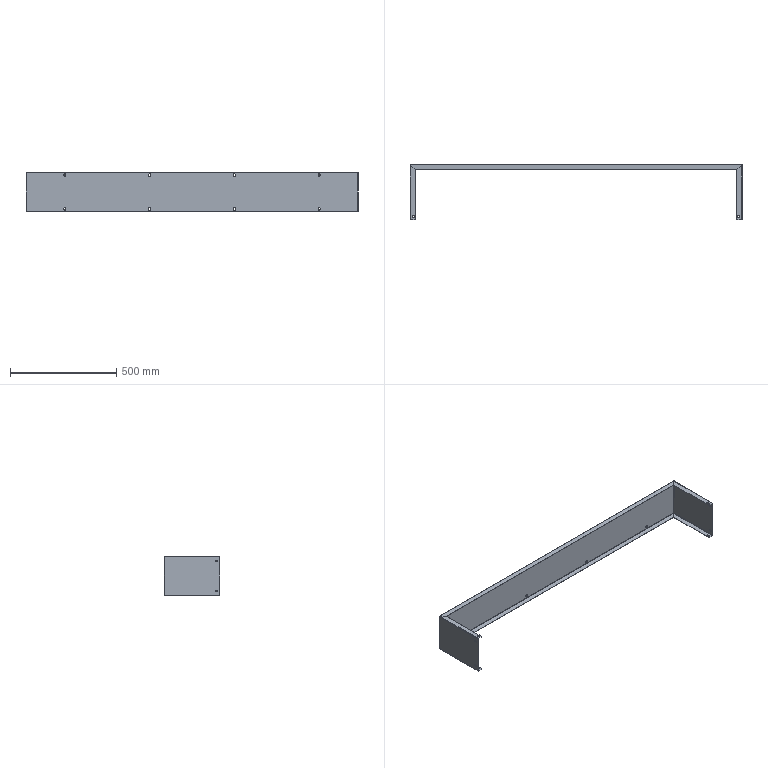Part | SolidWorks | features BaseBody 1 | 1 solid | 146 faces | box 1564 x 260 x 187.4 mm | volume 579055 mm3 | plane 78 | cylinder 60 | spline 8 | commonest cylinder face diameters 7 x40 2 x8 4.4 x8 10 x4